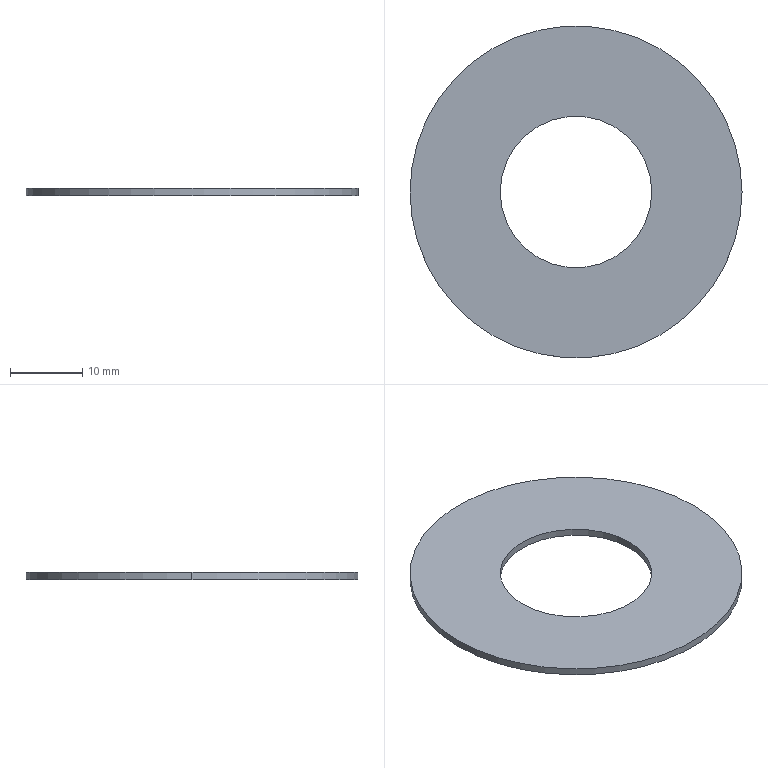Part | SolidWorks | features Extrusion 1 | 1 solid | 6 faces | box 46 x 46 x 1 mm | volume 1316 mm3 | cylinder 4 | plane 2 | commonest cylinder face diameters 21 x2 46 x2
STEP:
#1=CARTESIAN_POINT('',(-10.5,0.,1.));
#2=VERTEX_POINT('',#1);
#3=CARTESIAN_POINT('',(10.5,0.,1.));
#4=VERTEX_POINT('',#3);
#5=CARTESIAN_POINT('',(0.,0.,1.));
#6=DIRECTION('',(0.,0.,1.));
#7=DIRECTION('',(1.,0.,0.));
#8=AXIS2_PLACEMENT_3D('',#5,#6,#7);
#9=CIRCLE('',#8,10.5);
#10=EDGE_CURVE('',#2,#4,#9,.T.);
#11=ORIENTED_EDGE('',*,*,#10,.T.);
#12=CARTESIAN_POINT('',(10.5,0.,0.));
#13=VERTEX_POINT('',#12);
#14=CARTESIAN_POINT('',(10.5,0.,1.));
#15=DIRECTION('',(0.,0.,-1.));
#16=VECTOR('',#15,1000.);
#17=LINE('',#14,#16);
#18=EDGE_CURVE('',#4,#13,#17,.T.);
#19=ORIENTED_EDGE('',*,*,#18,.T.);
#20=CARTESIAN_POINT('',(-10.5,0.,0.));
#21=VERTEX_POINT('',#20);
#22=CARTESIAN_POINT('',(0.,0.,0.));
#23=DIRECTION('',(0.,0.,1.));
#24=DIRECTION('',(1.,0.,0.));
#25=AXIS2_PLACEMENT_3D('',#22,#23,#24);
#26=CIRCLE('',#25,10.5);
#27=EDGE_CURVE('',#21,#13,#26,.T.);
#28=ORIENTED_EDGE('',*,*,#27,.F.);
#29=CARTESIAN_POINT('',(-10.5,0.,1.));
#30=DIRECTION('',(0.,0.,-1.));
#31=VECTOR('',#30,1000.);
#32=LINE('',#29,#31);
#33=EDGE_CURVE('',#2,#21,#32,.T.);
#34=ORIENTED_EDGE('',*,*,#33,.F.);
#35=EDGE_LOOP('',(#11,#19,#28,#34));
#36=FACE_OUTER_BOUND('',#35,.T.);
#37=CARTESIAN_POINT('',(0.,0.,1.));
#38=DIRECTION('',(0.,0.,-1.));
#39=DIRECTION('',(-1.,0.,0.));
#40=AXIS2_PLACEMENT_3D('',#37,#38,#39);
#41=CYLINDRICAL_SURFACE('',#40,10.5);
#42=ADVANCED_FACE('',(#36),#41,.F.);
#43=CARTESIAN_POINT('',(23.,0.,1.));
#44=VERTEX_POINT('',#43);
#45=CARTESIAN_POINT('',(-23.,0.,1.));
#46=VERTEX_POINT('',#45);
#47=CARTESIAN_POINT('',(0.,0.,1.));
#48=DIRECTION('',(0.,0.,1.));
#49=DIRECTION('',(1.,0.,0.));
#50=AXIS2_PLACEMENT_3D('',#47,#48,#49);
#51=CIRCLE('',#50,23.);
#52=EDGE_CURVE('',#44,#46,#51,.T.);
#53=ORIENTED_EDGE('',*,*,#52,.F.);
#54=CARTESIAN_POINT('',(23.,0.,0.));
#55=VERTEX_POINT('',#54);
#56=CARTESIAN_POINT('',(23.,0.,1.));
#57=DIRECTION('',(0.,0.,-1.));
#58=VECTOR('',#57,1000.);
#59=LINE('',#56,#58);
#60=EDGE_CURVE('',#44,#55,#59,.T.);
#61=ORIENTED_EDGE('',*,*,#60,.T.);
#62=CARTESIAN_POINT('',(-23.,0.,0.));
#63=VERTEX_POINT('',#62);
#64=CARTESIAN_POINT('',(0.,0.,0.));
#65=DIRECTION('',(0.,0.,1.));
#66=DIRECTION('',(1.,0.,0.));
#67=AXIS2_PLACEMENT_3D('',#64,#65,#66);
#68=CIRCLE('',#67,23.);
#69=EDGE_CURVE('',#55,#63,#68,.T.);
#70=ORIENTED_EDGE('',*,*,#69,.T.);
#71=CARTESIAN_POINT('',(-23.,0.,1.));
#72=DIRECTION('',(0.,0.,-1.));
#73=VECTOR('',#72,1000.);
#74=LINE('',#71,#73);
#75=EDGE_CURVE('',#46,#63,#74,.T.);
#76=ORIENTED_EDGE('',*,*,#75,.F.);
#77=EDGE_LOOP('',(#53,#61,#70,#76));
#78=FACE_OUTER_BOUND('',#77,.T.);
#79=CARTESIAN_POINT('',(0.,0.,1.));
#80=DIRECTION('',(0.,0.,-1.));
#81=DIRECTION('',(-1.,0.,0.));
#82=AXIS2_PLACEMENT_3D('',#79,#80,#81);
#83=CYLINDRICAL_SURFACE('',#82,23.);
#84=ADVANCED_FACE('',(#78),#83,.T.);
#85=CARTESIAN_POINT('',(0.,0.,1.));
#86=DIRECTION('',(0.,0.,1.));
#87=DIRECTION('',(1.,0.,0.));
#88=AXIS2_PLACEMENT_3D('',#85,#86,#87);
#89=CIRCLE('',#88,23.);
#90=EDGE_CURVE('',#46,#44,#89,.T.);
#91=ORIENTED_EDGE('',*,*,#90,.T.);
#92=ORIENTED_EDGE('',*,*,#52,.T.);
#93=EDGE_LOOP('',(#91,#92));
#94=FACE_OUTER_BOUND('',#93,.T.);
#95=ORIENTED_EDGE('',*,*,#10,.F.);
#96=CARTESIAN_POINT('',(0.,0.,1.));
#97=DIRECTION('',(0.,0.,1.));
#98=DIRECTION('',(1.,0.,0.));
#99=AXIS2_PLACEMENT_3D('',#96,#97,#98);
#100=CIRCLE('',#99,10.5);
#101=EDGE_CURVE('',#4,#2,#100,.T.);
#102=ORIENTED_EDGE('',*,*,#101,.F.);
#103=EDGE_LOOP('',(#95,#102));
#104=FACE_BOUND('',#103,.T.);
#105=CARTESIAN_POINT('',(0.,0.,1.));
#106=DIRECTION('',(0.,0.,1.));
#107=DIRECTION('',(1.,0.,0.));
#108=AXIS2_PLACEMENT_3D('',#105,#106,#107);
#109=PLANE('',#108);
#110=ADVANCED_FACE('',(#94,#104),#109,.T.);
#111=CARTESIAN_POINT('',(0.,0.,0.));
#112=DIRECTION('',(0.,0.,1.));
#113=DIRECTION('',(1.,0.,0.));
#114=AXIS2_PLACEMENT_3D('',#111,#112,#113);
#115=CIRCLE('',#114,23.);
#116=EDGE_CURVE('',#63,#55,#115,.T.);
#117=ORIENTED_EDGE('',*,*,#116,.F.);
#118=ORIENTED_EDGE('',*,*,#69,.F.);
#119=EDGE_LOOP('',(#117,#118));
#120=FACE_OUTER_BOUND('',#119,.T.);
#121=ORIENTED_EDGE('',*,*,#27,.T.);
#122=CARTESIAN_POINT('',(0.,0.,0.));
#123=DIRECTION('',(0.,0.,1.));
#124=DIRECTION('',(1.,0.,0.));
#125=AXIS2_PLACEMENT_3D('',#122,#123,#124);
#126=CIRCLE('',#125,10.5);
#127=EDGE_CURVE('',#13,#21,#126,.T.);
#128=ORIENTED_EDGE('',*,*,#127,.T.);
#129=EDGE_LOOP('',(#121,#128));
#130=FACE_BOUND('',#129,.T.);
#131=CARTESIAN_POINT('',(0.,0.,0.));
#132=DIRECTION('',(0.,0.,1.));
#133=DIRECTION('',(1.,0.,0.));
#134=AXIS2_PLACEMENT_3D('',#131,#132,#133);
#135=PLANE('',#134);
#136=ADVANCED_FACE('',(#120,#130),#135,.F.);
#137=ORIENTED_EDGE('',*,*,#60,.F.);
#138=ORIENTED_EDGE('',*,*,#90,.F.);
#139=ORIENTED_EDGE('',*,*,#75,.T.);
#140=ORIENTED_EDGE('',*,*,#116,.T.);
#141=EDGE_LOOP('',(#137,#138,#139,#140));
#142=FACE_OUTER_BOUND('',#141,.T.);
#143=CARTESIAN_POINT('',(0.,0.,1.));
#144=DIRECTION('',(0.,0.,-1.));
#145=DIRECTION('',(-1.,0.,0.));
#146=AXIS2_PLACEMENT_3D('',#143,#144,#145);
#147=CYLINDRICAL_SURFACE('',#146,23.);
#148=ADVANCED_FACE('',(#142),#147,.T.);
#149=ORIENTED_EDGE('',*,*,#18,.F.);
#150=ORIENTED_EDGE('',*,*,#101,.T.);
#151=ORIENTED_EDGE('',*,*,#33,.T.);
#152=ORIENTED_EDGE('',*,*,#127,.F.);
#153=EDGE_LOOP('',(#149,#150,#151,#152));
#154=FACE_OUTER_BOUND('',#153,.T.);
#155=CARTESIAN_POINT('',(0.,0.,1.));
#156=DIRECTION('',(0.,0.,-1.));
#157=DIRECTION('',(-1.,0.,0.));
#158=AXIS2_PLACEMENT_3D('',#155,#156,#157);
#159=CYLINDRICAL_SURFACE('',#158,10.5);
#160=ADVANCED_FACE('',(#154),#159,.F.);
#161=CLOSED_SHELL('',(#42,#84,#110,#136,#148,#160));
#162=MANIFOLD_SOLID_BREP('',#161);
#163=CARTESIAN_POINT('',(0.,0.,0.));
#164=DIRECTION('',(0.,0.,1.));
#165=DIRECTION('',(1.,0.,0.));
#166=AXIS2_PLACEMENT_3D('',#163,#164,#165);
#167=(LENGTH_UNIT()NAMED_UNIT(*)SI_UNIT(.MILLI.,.METRE.));
#168=UNCERTAINTY_MEASURE_WITH_UNIT(LENGTH_MEASURE(0.00001),#167,'','');
#169=(NAMED_UNIT(*)PLANE_ANGLE_UNIT()SI_UNIT($,.RADIAN.));
#170=(NAMED_UNIT(*)SI_UNIT($,.STERADIAN.)SOLID_ANGLE_UNIT());
#171=(GEOMETRIC_REPRESENTATION_CONTEXT(3)GLOBAL_UNCERTAINTY_ASSIGNED_CONTEXT((#168))GLOBAL_UNIT_ASSIGNED_CONTEXT((#167,#169,#170))REPRESENTATION_CONTEXT('',''));
#172=ADVANCED_BREP_SHAPE_REPRESENTATION('',(#162,#166),#171);